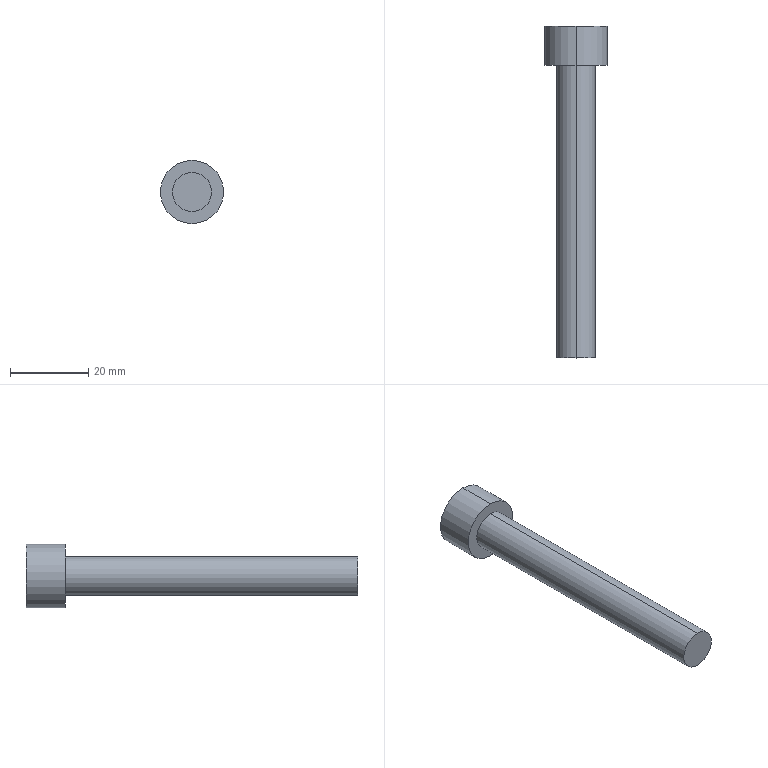Part | SolidWorks | features ICE 1, Revolution 1 | 1 solid | 14 faces | box 16.2 x 85 x 16.2 mm | volume 7619 mm3 | plane 10 | cylinder 4 | commonest cylinder face diameters 10 x2 16.2 x2
STEP:
#1=CARTESIAN_POINT('',(0.,-75.,5.));
#2=VERTEX_POINT('',#1);
#3=CARTESIAN_POINT('',(0.,-75.,-5.));
#4=VERTEX_POINT('',#3);
#5=CARTESIAN_POINT('',(0.,-75.,0.));
#6=DIRECTION('',(0.,1.,0.));
#7=DIRECTION('',(0.,0.,1.));
#8=AXIS2_PLACEMENT_3D('',#5,#6,#7);
#9=CIRCLE('',#8,5.);
#10=EDGE_CURVE('',#2,#4,#9,.T.);
#11=ORIENTED_EDGE('',*,*,#10,.T.);
#12=CARTESIAN_POINT('',(0.,0.,-5.));
#13=VERTEX_POINT('',#12);
#14=CARTESIAN_POINT('',(0.,11.322,-5.));
#15=DIRECTION('',(0.,1.,0.));
#16=VECTOR('',#15,1000.);
#17=LINE('',#14,#16);
#18=EDGE_CURVE('',#4,#13,#17,.T.);
#19=ORIENTED_EDGE('',*,*,#18,.T.);
#20=CARTESIAN_POINT('',(0.,0.,5.));
#21=VERTEX_POINT('',#20);
#22=CARTESIAN_POINT('',(0.,0.,0.));
#23=DIRECTION('',(0.,1.,0.));
#24=DIRECTION('',(0.,0.,1.));
#25=AXIS2_PLACEMENT_3D('',#22,#23,#24);
#26=CIRCLE('',#25,5.);
#27=EDGE_CURVE('',#21,#13,#26,.T.);
#28=ORIENTED_EDGE('',*,*,#27,.F.);
#29=CARTESIAN_POINT('',(0.,11.322,5.));
#30=DIRECTION('',(0.,1.,0.));
#31=VECTOR('',#30,1000.);
#32=LINE('',#29,#31);
#33=EDGE_CURVE('',#2,#21,#32,.T.);
#34=ORIENTED_EDGE('',*,*,#33,.F.);
#35=EDGE_LOOP('',(#11,#19,#28,#34));
#36=FACE_OUTER_BOUND('',#35,.T.);
#37=CARTESIAN_POINT('',(0.,11.322,0.));
#38=DIRECTION('',(0.,1.,0.));
#39=DIRECTION('',(0.,0.,1.));
#40=AXIS2_PLACEMENT_3D('',#37,#38,#39);
#41=CYLINDRICAL_SURFACE('',#40,5.);
#42=ADVANCED_FACE('',(#36),#41,.T.);
#43=CARTESIAN_POINT('',(0.,0.,8.1));
#44=VERTEX_POINT('',#43);
#45=CARTESIAN_POINT('',(0.,0.,-8.1));
#46=VERTEX_POINT('',#45);
#47=CARTESIAN_POINT('',(0.,0.,0.));
#48=DIRECTION('',(0.,1.,0.));
#49=DIRECTION('',(0.,0.,1.));
#50=AXIS2_PLACEMENT_3D('',#47,#48,#49);
#51=CIRCLE('',#50,8.1);
#52=EDGE_CURVE('',#44,#46,#51,.T.);
#53=ORIENTED_EDGE('',*,*,#52,.T.);
#54=CARTESIAN_POINT('',(0.,10.,-8.1));
#55=VERTEX_POINT('',#54);
#56=CARTESIAN_POINT('',(0.,11.322,-8.1));
#57=DIRECTION('',(0.,1.,0.));
#58=VECTOR('',#57,1000.);
#59=LINE('',#56,#58);
#60=EDGE_CURVE('',#46,#55,#59,.T.);
#61=ORIENTED_EDGE('',*,*,#60,.T.);
#62=CARTESIAN_POINT('',(0.,10.,8.1));
#63=VERTEX_POINT('',#62);
#64=CARTESIAN_POINT('',(0.,10.,0.));
#65=DIRECTION('',(0.,1.,0.));
#66=DIRECTION('',(0.,0.,1.));
#67=AXIS2_PLACEMENT_3D('',#64,#65,#66);
#68=CIRCLE('',#67,8.1);
#69=EDGE_CURVE('',#63,#55,#68,.T.);
#70=ORIENTED_EDGE('',*,*,#69,.F.);
#71=CARTESIAN_POINT('',(0.,11.322,8.1));
#72=DIRECTION('',(0.,1.,0.));
#73=VECTOR('',#72,1000.);
#74=LINE('',#71,#73);
#75=EDGE_CURVE('',#44,#63,#74,.T.);
#76=ORIENTED_EDGE('',*,*,#75,.F.);
#77=EDGE_LOOP('',(#53,#61,#70,#76));
#78=FACE_OUTER_BOUND('',#77,.T.);
#79=CARTESIAN_POINT('',(0.,11.322,0.));
#80=DIRECTION('',(0.,1.,0.));
#81=DIRECTION('',(0.,0.,1.));
#82=AXIS2_PLACEMENT_3D('',#79,#80,#81);
#83=CYLINDRICAL_SURFACE('',#82,8.1);
#84=ADVANCED_FACE('',(#78),#83,.T.);
#85=CARTESIAN_POINT('',(4.,10.,-2.309));
#86=VERTEX_POINT('',#85);
#87=CARTESIAN_POINT('',(0.,10.,-4.619));
#88=VERTEX_POINT('',#87);
#89=CARTESIAN_POINT('',(4.,10.,-2.309));
#90=DIRECTION('',(-0.866,0.,-0.5));
#91=VECTOR('',#90,1000.);
#92=LINE('',#89,#91);
#93=EDGE_CURVE('',#86,#88,#92,.T.);
#94=ORIENTED_EDGE('',*,*,#93,.F.);
#95=CARTESIAN_POINT('',(4.,10.,2.309));
#96=VERTEX_POINT('',#95);
#97=CARTESIAN_POINT('',(4.,10.,2.309));
#98=DIRECTION('',(0.,0.,-1.));
#99=VECTOR('',#98,1000.);
#100=LINE('',#97,#99);
#101=EDGE_CURVE('',#96,#86,#100,.T.);
#102=ORIENTED_EDGE('',*,*,#101,.F.);
#103=CARTESIAN_POINT('',(0.,10.,4.619));
#104=VERTEX_POINT('',#103);
#105=CARTESIAN_POINT('',(0.,10.,4.619));
#106=DIRECTION('',(0.866,0.,-0.5));
#107=VECTOR('',#106,1000.);
#108=LINE('',#105,#107);
#109=EDGE_CURVE('',#104,#96,#108,.T.);
#110=ORIENTED_EDGE('',*,*,#109,.F.);
#111=CARTESIAN_POINT('',(-4.,10.,2.309));
#112=VERTEX_POINT('',#111);
#113=CARTESIAN_POINT('',(-4.,10.,2.309));
#114=DIRECTION('',(0.866,0.,0.5));
#115=VECTOR('',#114,1000.);
#116=LINE('',#113,#115);
#117=EDGE_CURVE('',#112,#104,#116,.T.);
#118=ORIENTED_EDGE('',*,*,#117,.F.);
#119=CARTESIAN_POINT('',(-4.,10.,-2.309));
#120=VERTEX_POINT('',#119);
#121=CARTESIAN_POINT('',(-4.,10.,-2.309));
#122=DIRECTION('',(0.,0.,1.));
#123=VECTOR('',#122,1000.);
#124=LINE('',#121,#123);
#125=EDGE_CURVE('',#120,#112,#124,.T.);
#126=ORIENTED_EDGE('',*,*,#125,.F.);
#127=CARTESIAN_POINT('',(0.,10.,-4.619));
#128=DIRECTION('',(-0.866,0.,0.5));
#129=VECTOR('',#128,1000.);
#130=LINE('',#127,#129);
#131=EDGE_CURVE('',#88,#120,#130,.T.);
#132=ORIENTED_EDGE('',*,*,#131,.F.);
#133=EDGE_LOOP('',(#94,#102,#110,#118,#126,#132));
#134=FACE_BOUND('',#133,.T.);
#135=ORIENTED_EDGE('',*,*,#69,.T.);
#136=CARTESIAN_POINT('',(0.,10.,0.));
#137=DIRECTION('',(0.,1.,0.));
#138=DIRECTION('',(0.,0.,1.));
#139=AXIS2_PLACEMENT_3D('',#136,#137,#138);
#140=CIRCLE('',#139,8.1);
#141=EDGE_CURVE('',#55,#63,#140,.T.);
#142=ORIENTED_EDGE('',*,*,#141,.T.);
#143=EDGE_LOOP('',(#135,#142));
#144=FACE_OUTER_BOUND('',#143,.T.);
#145=CARTESIAN_POINT('',(0.,10.,0.));
#146=DIRECTION('',(0.,1.,0.));
#147=DIRECTION('',(0.,0.,1.));
#148=AXIS2_PLACEMENT_3D('',#145,#146,#147);
#149=PLANE('',#148);
#150=ADVANCED_FACE('',(#134,#144),#149,.T.);
#151=ORIENTED_EDGE('',*,*,#60,.F.);
#152=CARTESIAN_POINT('',(0.,0.,0.));
#153=DIRECTION('',(0.,1.,0.));
#154=DIRECTION('',(0.,0.,1.));
#155=AXIS2_PLACEMENT_3D('',#152,#153,#154);
#156=CIRCLE('',#155,8.1);
#157=EDGE_CURVE('',#46,#44,#156,.T.);
#158=ORIENTED_EDGE('',*,*,#157,.T.);
#159=ORIENTED_EDGE('',*,*,#75,.T.);
#160=ORIENTED_EDGE('',*,*,#141,.F.);
#161=EDGE_LOOP('',(#151,#158,#159,#160));
#162=FACE_OUTER_BOUND('',#161,.T.);
#163=CARTESIAN_POINT('',(0.,11.322,0.));
#164=DIRECTION('',(0.,1.,0.));
#165=DIRECTION('',(0.,0.,1.));
#166=AXIS2_PLACEMENT_3D('',#163,#164,#165);
#167=CYLINDRICAL_SURFACE('',#166,8.1);
#168=ADVANCED_FACE('',(#162),#167,.T.);
#169=ORIENTED_EDGE('',*,*,#27,.T.);
#170=CARTESIAN_POINT('',(0.,0.,0.));
#171=DIRECTION('',(0.,1.,0.));
#172=DIRECTION('',(0.,0.,1.));
#173=AXIS2_PLACEMENT_3D('',#170,#171,#172);
#174=CIRCLE('',#173,5.);
#175=EDGE_CURVE('',#13,#21,#174,.T.);
#176=ORIENTED_EDGE('',*,*,#175,.T.);
#177=EDGE_LOOP('',(#169,#176));
#178=FACE_BOUND('',#177,.T.);
#179=ORIENTED_EDGE('',*,*,#52,.F.);
#180=ORIENTED_EDGE('',*,*,#157,.F.);
#181=EDGE_LOOP('',(#179,#180));
#182=FACE_OUTER_BOUND('',#181,.T.);
#183=CARTESIAN_POINT('',(-8.1,0.,0.));
#184=DIRECTION('',(0.,-1.,0.));
#185=DIRECTION('',(0.,0.,-1.));
#186=AXIS2_PLACEMENT_3D('',#183,#184,#185);
#187=PLANE('',#186);
#188=ADVANCED_FACE('',(#178,#182),#187,.T.);
#189=ORIENTED_EDGE('',*,*,#18,.F.);
#190=CARTESIAN_POINT('',(0.,-75.,0.));
#191=DIRECTION('',(0.,1.,0.));
#192=DIRECTION('',(0.,0.,1.));
#193=AXIS2_PLACEMENT_3D('',#190,#191,#192);
#194=CIRCLE('',#193,5.);
#195=EDGE_CURVE('',#4,#2,#194,.T.);
#196=ORIENTED_EDGE('',*,*,#195,.T.);
#197=ORIENTED_EDGE('',*,*,#33,.T.);
#198=ORIENTED_EDGE('',*,*,#175,.F.);
#199=EDGE_LOOP('',(#189,#196,#197,#198));
#200=FACE_OUTER_BOUND('',#199,.T.);
#201=CARTESIAN_POINT('',(0.,11.322,0.));
#202=DIRECTION('',(0.,1.,0.));
#203=DIRECTION('',(0.,0.,1.));
#204=AXIS2_PLACEMENT_3D('',#201,#202,#203);
#205=CYLINDRICAL_SURFACE('',#204,5.);
#206=ADVANCED_FACE('',(#200),#205,.T.);
#207=ORIENTED_EDGE('',*,*,#10,.F.);
#208=ORIENTED_EDGE('',*,*,#195,.F.);
#209=EDGE_LOOP('',(#207,#208));
#210=FACE_OUTER_BOUND('',#209,.T.);
#211=CARTESIAN_POINT('',(-5.,-75.,0.));
#212=DIRECTION('',(0.,-1.,0.));
#213=DIRECTION('',(0.,0.,-1.));
#214=AXIS2_PLACEMENT_3D('',#211,#212,#213);
#215=PLANE('',#214);
#216=ADVANCED_FACE('',(#210),#215,.T.);
#217=ORIENTED_EDGE('',*,*,#93,.T.);
#218=CARTESIAN_POINT('',(0.,4.,-4.619));
#219=VERTEX_POINT('',#218);
#220=CARTESIAN_POINT('',(0.,4.,-4.619));
#221=DIRECTION('',(0.,1.,0.));
#222=VECTOR('',#221,1000.);
#223=LINE('',#220,#222);
#224=EDGE_CURVE('',#219,#88,#223,.T.);
#225=ORIENTED_EDGE('',*,*,#224,.F.);
#226=CARTESIAN_POINT('',(4.,4.,-2.309));
#227=VERTEX_POINT('',#226);
#228=CARTESIAN_POINT('',(4.,4.,-2.309));
#229=DIRECTION('',(-0.866,0.,-0.5));
#230=VECTOR('',#229,1000.);
#231=LINE('',#228,#230);
#232=EDGE_CURVE('',#227,#219,#231,.T.);
#233=ORIENTED_EDGE('',*,*,#232,.F.);
#234=CARTESIAN_POINT('',(4.,4.,-2.309));
#235=DIRECTION('',(0.,1.,0.));
#236=VECTOR('',#235,1000.);
#237=LINE('',#234,#236);
#238=EDGE_CURVE('',#227,#86,#237,.T.);
#239=ORIENTED_EDGE('',*,*,#238,.T.);
#240=EDGE_LOOP('',(#217,#225,#233,#239));
#241=FACE_OUTER_BOUND('',#240,.T.);
#242=CARTESIAN_POINT('',(4.,4.,-2.309));
#243=DIRECTION('',(0.5,0.,-0.866));
#244=DIRECTION('',(-0.866,0.,-0.5));
#245=AXIS2_PLACEMENT_3D('',#242,#243,#244);
#246=PLANE('',#245);
#247=ADVANCED_FACE('',(#241),#246,.F.);
#248=ORIENTED_EDGE('',*,*,#101,.T.);
#249=ORIENTED_EDGE('',*,*,#238,.F.);
#250=CARTESIAN_POINT('',(4.,4.,2.309));
#251=VERTEX_POINT('',#250);
#252=CARTESIAN_POINT('',(4.,4.,2.309));
#253=DIRECTION('',(0.,0.,-1.));
#254=VECTOR('',#253,1000.);
#255=LINE('',#252,#254);
#256=EDGE_CURVE('',#251,#227,#255,.T.);
#257=ORIENTED_EDGE('',*,*,#256,.F.);
#258=CARTESIAN_POINT('',(4.,4.,2.309));
#259=DIRECTION('',(0.,1.,0.));
#260=VECTOR('',#259,1000.);
#261=LINE('',#258,#260);
#262=EDGE_CURVE('',#251,#96,#261,.T.);
#263=ORIENTED_EDGE('',*,*,#262,.T.);
#264=EDGE_LOOP('',(#248,#249,#257,#263));
#265=FACE_OUTER_BOUND('',#264,.T.);
#266=CARTESIAN_POINT('',(4.,4.,2.309));
#267=DIRECTION('',(1.,0.,0.));
#268=DIRECTION('',(0.,0.,-1.));
#269=AXIS2_PLACEMENT_3D('',#266,#267,#268);
#270=PLANE('',#269);
#271=ADVANCED_FACE('',(#265),#270,.F.);
#272=ORIENTED_EDGE('',*,*,#109,.T.);
#273=ORIENTED_EDGE('',*,*,#262,.F.);
#274=CARTESIAN_POINT('',(0.,4.,4.619));
#275=VERTEX_POINT('',#274);
#276=CARTESIAN_POINT('',(0.,4.,4.619));
#277=DIRECTION('',(0.866,0.,-0.5));
#278=VECTOR('',#277,1000.);
#279=LINE('',#276,#278);
#280=EDGE_CURVE('',#275,#251,#279,.T.);
#281=ORIENTED_EDGE('',*,*,#280,.F.);
#282=CARTESIAN_POINT('',(0.,4.,4.619));
#283=DIRECTION('',(0.,1.,0.));
#284=VECTOR('',#283,1000.);
#285=LINE('',#282,#284);
#286=EDGE_CURVE('',#275,#104,#285,.T.);
#287=ORIENTED_EDGE('',*,*,#286,.T.);
#288=EDGE_LOOP('',(#272,#273,#281,#287));
#289=FACE_OUTER_BOUND('',#288,.T.);
#290=CARTESIAN_POINT('',(0.,4.,4.619));
#291=DIRECTION('',(0.5,0.,0.866));
#292=DIRECTION('',(0.866,0.,-0.5));
#293=AXIS2_PLACEMENT_3D('',#290,#291,#292);
#294=PLANE('',#293);
#295=ADVANCED_FACE('',(#289),#294,.F.);
#296=ORIENTED_EDGE('',*,*,#117,.T.);
#297=ORIENTED_EDGE('',*,*,#286,.F.);
#298=CARTESIAN_POINT('',(-4.,4.,2.309));
#299=VERTEX_POINT('',#298);
#300=CARTESIAN_POINT('',(-4.,4.,2.309));
#301=DIRECTION('',(0.866,0.,0.5));
#302=VECTOR('',#301,1000.);
#303=LINE('',#300,#302);
#304=EDGE_CURVE('',#299,#275,#303,.T.);
#305=ORIENTED_EDGE('',*,*,#304,.F.);
#306=CARTESIAN_POINT('',(-4.,4.,2.309));
#307=DIRECTION('',(0.,1.,0.));
#308=VECTOR('',#307,1000.);
#309=LINE('',#306,#308);
#310=EDGE_CURVE('',#299,#112,#309,.T.);
#311=ORIENTED_EDGE('',*,*,#310,.T.);
#312=EDGE_LOOP('',(#296,#297,#305,#311));
#313=FACE_OUTER_BOUND('',#312,.T.);
#314=CARTESIAN_POINT('',(-4.,4.,2.309));
#315=DIRECTION('',(-0.5,0.,0.866));
#316=DIRECTION('',(0.866,0.,0.5));
#317=AXIS2_PLACEMENT_3D('',#314,#315,#316);
#318=PLANE('',#317);
#319=ADVANCED_FACE('',(#313),#318,.F.);
#320=ORIENTED_EDGE('',*,*,#125,.T.);
#321=ORIENTED_EDGE('',*,*,#310,.F.);
#322=CARTESIAN_POINT('',(-4.,4.,-2.309));
#323=VERTEX_POINT('',#322);
#324=CARTESIAN_POINT('',(-4.,4.,-2.309));
#325=DIRECTION('',(0.,0.,1.));
#326=VECTOR('',#325,1000.);
#327=LINE('',#324,#326);
#328=EDGE_CURVE('',#323,#299,#327,.T.);
#329=ORIENTED_EDGE('',*,*,#328,.F.);
#330=CARTESIAN_POINT('',(-4.,4.,-2.309));
#331=DIRECTION('',(0.,1.,0.));
#332=VECTOR('',#331,1000.);
#333=LINE('',#330,#332);
#334=EDGE_CURVE('',#323,#120,#333,.T.);
#335=ORIENTED_EDGE('',*,*,#334,.T.);
#336=EDGE_LOOP('',(#320,#321,#329,#335));
#337=FACE_OUTER_BOUND('',#336,.T.);
#338=CARTESIAN_POINT('',(-4.,4.,-2.309));
#339=DIRECTION('',(-1.,0.,0.));
#340=DIRECTION('',(0.,0.,1.));
#341=AXIS2_PLACEMENT_3D('',#338,#339,#340);
#342=PLANE('',#341);
#343=ADVANCED_FACE('',(#337),#342,.F.);
#344=ORIENTED_EDGE('',*,*,#131,.T.);
#345=ORIENTED_EDGE('',*,*,#334,.F.);
#346=CARTESIAN_POINT('',(0.,4.,-4.619));
#347=DIRECTION('',(-0.866,0.,0.5));
#348=VECTOR('',#347,1000.);
#349=LINE('',#346,#348);
#350=EDGE_CURVE('',#219,#323,#349,.T.);
#351=ORIENTED_EDGE('',*,*,#350,.F.);
#352=ORIENTED_EDGE('',*,*,#224,.T.);
#353=EDGE_LOOP('',(#344,#345,#351,#352));
#354=FACE_OUTER_BOUND('',#353,.T.);
#355=CARTESIAN_POINT('',(0.,4.,-4.619));
#356=DIRECTION('',(-0.5,0.,-0.866));
#357=DIRECTION('',(-0.866,0.,0.5));
#358=AXIS2_PLACEMENT_3D('',#355,#356,#357);
#359=PLANE('',#358);
#360=ADVANCED_FACE('',(#354),#359,.F.);
#361=ORIENTED_EDGE('',*,*,#232,.T.);
#362=ORIENTED_EDGE('',*,*,#350,.T.);
#363=ORIENTED_EDGE('',*,*,#328,.T.);
#364=ORIENTED_EDGE('',*,*,#304,.T.);
#365=ORIENTED_EDGE('',*,*,#280,.T.);
#366=ORIENTED_EDGE('',*,*,#256,.T.);
#367=EDGE_LOOP('',(#361,#362,#363,#364,#365,#366));
#368=FACE_OUTER_BOUND('',#367,.T.);
#369=CARTESIAN_POINT('',(0.,4.,0.));
#370=DIRECTION('',(0.,1.,0.));
#371=DIRECTION('',(0.,0.,1.));
#372=AXIS2_PLACEMENT_3D('',#369,#370,#371);
#373=PLANE('',#372);
#374=ADVANCED_FACE('',(#368),#373,.T.);
#375=CLOSED_SHELL('',(#42,#84,#150,#168,#188,#206,#216,#247,#271,#295,#319,#343,#360,#374));
#376=MANIFOLD_SOLID_BREP('',#375);
#377=CARTESIAN_POINT('',(0.,0.,0.));
#378=DIRECTION('',(0.,0.,1.));
#379=DIRECTION('',(1.,0.,0.));
#380=AXIS2_PLACEMENT_3D('',#377,#378,#379);
#381=(LENGTH_UNIT()NAMED_UNIT(*)SI_UNIT(.MILLI.,.METRE.));
#382=UNCERTAINTY_MEASURE_WITH_UNIT(LENGTH_MEASURE(0.00001),#381,'','');
#383=(NAMED_UNIT(*)PLANE_ANGLE_UNIT()SI_UNIT($,.RADIAN.));
#384=(NAMED_UNIT(*)SI_UNIT($,.STERADIAN.)SOLID_ANGLE_UNIT());
#385=(GEOMETRIC_REPRESENTATION_CONTEXT(3)GLOBAL_UNCERTAINTY_ASSIGNED_CONTEXT((#382))GLOBAL_UNIT_ASSIGNED_CONTEXT((#381,#383,#384))REPRESENTATION_CONTEXT('',''));
#386=ADVANCED_BREP_SHAPE_REPRESENTATION('',(#376,#380),#385);